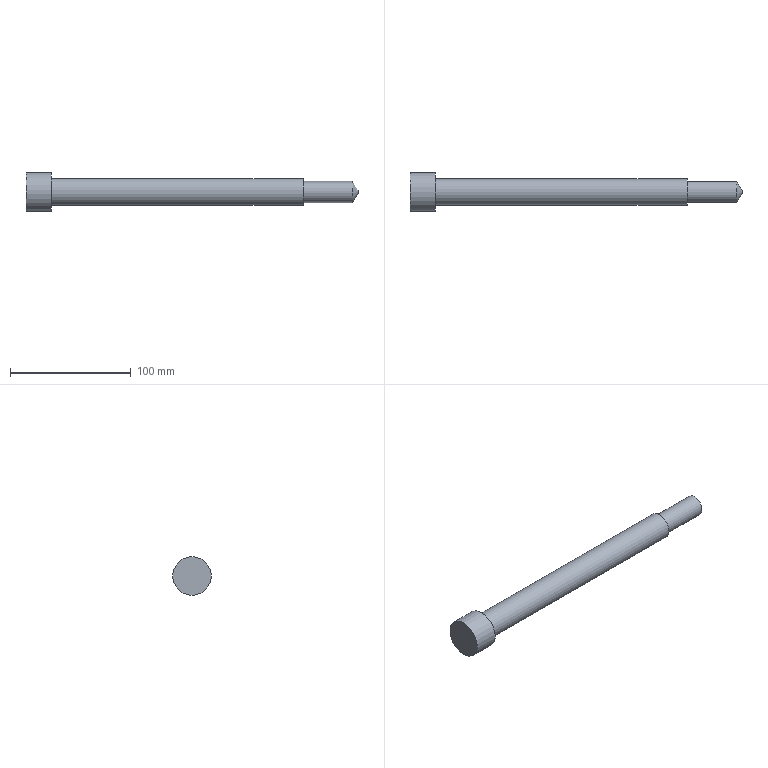Part | STEP file | solid 75 | 1 solid | 8 faces | box 275.5 x 32 x 32 mm | volume 106603 mm3 | plane 4 | cylinder 3 | cone 1 | commonest cylinder face diameters 17.5 x1 22 x1 32 x1